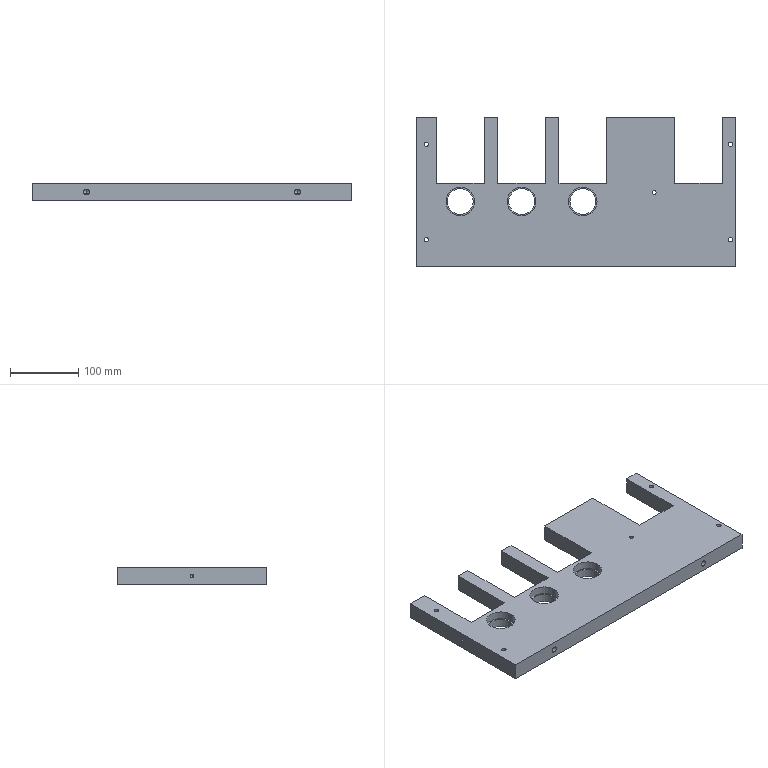Part | SolidWorks | features ICE 8, HoleWzd 3, LPattern 2, 3DProfileFeature 1, Extrusion 1 | 1 solid | 102 faces | box 470 x 220 x 25 mm | volume 1796756 mm3 | cylinder 52 | plane 30 | cone 20 | commonest cylinder face diameters 6.8 x12 6.5 x8 11 x8 38 x6 42 x6 5 x4